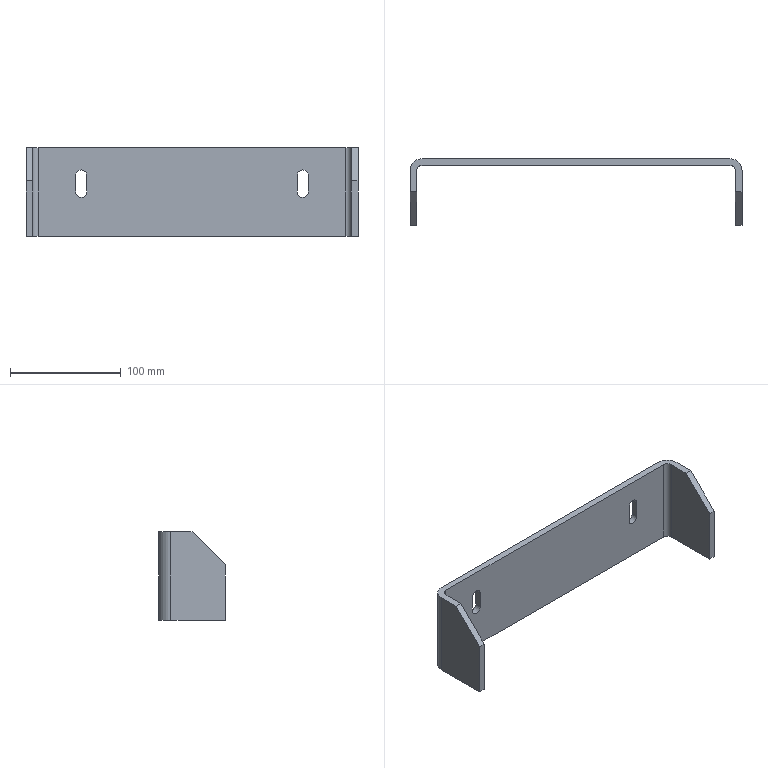Part | STEP file | VD-SYL0380DJ1006_1_1-12_VD-SYL0 | 1 solid | 26 faces | box 300 x 60 x 80 mm | volume 184401 mm3 | plane 16 | cylinder 10 | commonest cylinder face diameters 10 x8 22 x2
STEP:
#1=CARTESIAN_POINT('',(-105.,24.,15.));
#2=VERTEX_POINT('',#1);
#3=CARTESIAN_POINT('',(-100.,24.,20.));
#4=VERTEX_POINT('',#3);
#5=CARTESIAN_POINT('',(-100.,24.,15.));
#6=DIRECTION('',(0.,1.,0.));
#7=DIRECTION('',(-1.,0.,0.));
#8=AXIS2_PLACEMENT_3D('',#5,#6,#7);
#9=CIRCLE('',#8,5.);
#10=EDGE_CURVE('',#2,#4,#9,.T.);
#11=ORIENTED_EDGE('',*,*,#10,.F.);
#12=CARTESIAN_POINT('',(-105.,30.,15.));
#13=VERTEX_POINT('',#12);
#14=CARTESIAN_POINT('',(-105.,24.,15.));
#15=DIRECTION('',(0.,1.,0.));
#16=VECTOR('',#15,1000.);
#17=LINE('',#14,#16);
#18=EDGE_CURVE('',#2,#13,#17,.T.);
#19=ORIENTED_EDGE('',*,*,#18,.T.);
#20=CARTESIAN_POINT('',(-100.,30.,20.));
#21=VERTEX_POINT('',#20);
#22=CARTESIAN_POINT('',(-100.,30.,15.));
#23=DIRECTION('',(0.,-1.,0.));
#24=DIRECTION('',(0.,0.,1.));
#25=AXIS2_PLACEMENT_3D('',#22,#23,#24);
#26=CIRCLE('',#25,5.);
#27=EDGE_CURVE('',#21,#13,#26,.T.);
#28=ORIENTED_EDGE('',*,*,#27,.F.);
#29=CARTESIAN_POINT('',(-100.,30.,20.));
#30=DIRECTION('',(0.,-1.,0.));
#31=VECTOR('',#30,1000.);
#32=LINE('',#29,#31);
#33=EDGE_CURVE('',#21,#4,#32,.T.);
#34=ORIENTED_EDGE('',*,*,#33,.T.);
#35=EDGE_LOOP('',(#11,#19,#28,#34));
#36=FACE_OUTER_BOUND('',#35,.T.);
#37=CARTESIAN_POINT('',(-100.,27.,15.));
#38=DIRECTION('',(0.,1.,0.));
#39=DIRECTION('',(0.,0.,1.));
#40=AXIS2_PLACEMENT_3D('',#37,#38,#39);
#41=CYLINDRICAL_SURFACE('',#40,5.);
#42=ADVANCED_FACE('',(#36),#41,.F.);
#43=ORIENTED_EDGE('',*,*,#33,.F.);
#44=CARTESIAN_POINT('',(-95.,30.,15.));
#45=VERTEX_POINT('',#44);
#46=CARTESIAN_POINT('',(-100.,30.,15.));
#47=DIRECTION('',(0.,-1.,0.));
#48=DIRECTION('',(1.,0.,0.));
#49=AXIS2_PLACEMENT_3D('',#46,#47,#48);
#50=CIRCLE('',#49,5.);
#51=EDGE_CURVE('',#45,#21,#50,.T.);
#52=ORIENTED_EDGE('',*,*,#51,.F.);
#53=CARTESIAN_POINT('',(-95.,24.,15.));
#54=VERTEX_POINT('',#53);
#55=CARTESIAN_POINT('',(-95.,30.,15.));
#56=DIRECTION('',(0.,-1.,0.));
#57=VECTOR('',#56,1000.);
#58=LINE('',#55,#57);
#59=EDGE_CURVE('',#45,#54,#58,.T.);
#60=ORIENTED_EDGE('',*,*,#59,.T.);
#61=CARTESIAN_POINT('',(-100.,24.,15.));
#62=DIRECTION('',(0.,1.,0.));
#63=DIRECTION('',(0.,0.,1.));
#64=AXIS2_PLACEMENT_3D('',#61,#62,#63);
#65=CIRCLE('',#64,5.);
#66=EDGE_CURVE('',#4,#54,#65,.T.);
#67=ORIENTED_EDGE('',*,*,#66,.F.);
#68=EDGE_LOOP('',(#43,#52,#60,#67));
#69=FACE_OUTER_BOUND('',#68,.T.);
#70=CARTESIAN_POINT('',(-100.,27.,15.));
#71=DIRECTION('',(0.,1.,0.));
#72=DIRECTION('',(0.,0.,1.));
#73=AXIS2_PLACEMENT_3D('',#70,#71,#72);
#74=CYLINDRICAL_SURFACE('',#73,5.);
#75=ADVANCED_FACE('',(#69),#74,.F.);
#76=CARTESIAN_POINT('',(-95.,30.,0.));
#77=VERTEX_POINT('',#76);
#78=CARTESIAN_POINT('',(-95.,30.,15.));
#79=DIRECTION('',(0.,0.,-1.));
#80=VECTOR('',#79,1000.);
#81=LINE('',#78,#80);
#82=EDGE_CURVE('',#45,#77,#81,.T.);
#83=ORIENTED_EDGE('',*,*,#82,.T.);
#84=CARTESIAN_POINT('',(-95.,24.,0.));
#85=VERTEX_POINT('',#84);
#86=CARTESIAN_POINT('',(-95.,24.,0.));
#87=DIRECTION('',(0.,1.,0.));
#88=VECTOR('',#87,1000.);
#89=LINE('',#86,#88);
#90=EDGE_CURVE('',#85,#77,#89,.T.);
#91=ORIENTED_EDGE('',*,*,#90,.F.);
#92=CARTESIAN_POINT('',(-95.,24.,15.));
#93=DIRECTION('',(0.,0.,-1.));
#94=VECTOR('',#93,1000.);
#95=LINE('',#92,#94);
#96=EDGE_CURVE('',#54,#85,#95,.T.);
#97=ORIENTED_EDGE('',*,*,#96,.F.);
#98=ORIENTED_EDGE('',*,*,#59,.F.);
#99=EDGE_LOOP('',(#83,#91,#97,#98));
#100=FACE_OUTER_BOUND('',#99,.T.);
#101=CARTESIAN_POINT('',(-95.,27.,7.5));
#102=DIRECTION('',(-1.,0.,0.));
#103=DIRECTION('',(0.,0.,1.));
#104=AXIS2_PLACEMENT_3D('',#101,#102,#103);
#105=PLANE('',#104);
#106=ADVANCED_FACE('',(#100),#105,.T.);
#107=CARTESIAN_POINT('',(-105.,24.,0.));
#108=VERTEX_POINT('',#107);
#109=CARTESIAN_POINT('',(-100.,24.,0.));
#110=DIRECTION('',(0.,1.,0.));
#111=DIRECTION('',(1.,0.,0.));
#112=AXIS2_PLACEMENT_3D('',#109,#110,#111);
#113=CIRCLE('',#112,5.);
#114=EDGE_CURVE('',#85,#108,#113,.T.);
#115=ORIENTED_EDGE('',*,*,#114,.F.);
#116=ORIENTED_EDGE('',*,*,#90,.T.);
#117=CARTESIAN_POINT('',(-105.,30.,0.));
#118=VERTEX_POINT('',#117);
#119=CARTESIAN_POINT('',(-100.,30.,0.));
#120=DIRECTION('',(0.,-1.,0.));
#121=DIRECTION('',(-1.,0.,0.));
#122=AXIS2_PLACEMENT_3D('',#119,#120,#121);
#123=CIRCLE('',#122,5.);
#124=EDGE_CURVE('',#118,#77,#123,.T.);
#125=ORIENTED_EDGE('',*,*,#124,.F.);
#126=CARTESIAN_POINT('',(-105.,30.,0.));
#127=DIRECTION('',(0.,-1.,0.));
#128=VECTOR('',#127,1000.);
#129=LINE('',#126,#128);
#130=EDGE_CURVE('',#118,#108,#129,.T.);
#131=ORIENTED_EDGE('',*,*,#130,.T.);
#132=EDGE_LOOP('',(#115,#116,#125,#131));
#133=FACE_OUTER_BOUND('',#132,.T.);
#134=CARTESIAN_POINT('',(-100.,27.,0.));
#135=DIRECTION('',(0.,1.,0.));
#136=DIRECTION('',(0.,0.,1.));
#137=AXIS2_PLACEMENT_3D('',#134,#135,#136);
#138=CYLINDRICAL_SURFACE('',#137,5.);
#139=ADVANCED_FACE('',(#133),#138,.F.);
#140=CARTESIAN_POINT('',(-105.,30.,0.));
#141=DIRECTION('',(0.,0.,1.));
#142=VECTOR('',#141,1000.);
#143=LINE('',#140,#142);
#144=EDGE_CURVE('',#118,#13,#143,.T.);
#145=ORIENTED_EDGE('',*,*,#144,.T.);
#146=ORIENTED_EDGE('',*,*,#18,.F.);
#147=CARTESIAN_POINT('',(-105.,24.,0.));
#148=DIRECTION('',(0.,0.,1.));
#149=VECTOR('',#148,1000.);
#150=LINE('',#147,#149);
#151=EDGE_CURVE('',#108,#2,#150,.T.);
#152=ORIENTED_EDGE('',*,*,#151,.F.);
#153=ORIENTED_EDGE('',*,*,#130,.F.);
#154=EDGE_LOOP('',(#145,#146,#152,#153));
#155=FACE_OUTER_BOUND('',#154,.T.);
#156=CARTESIAN_POINT('',(-105.,27.,7.5));
#157=DIRECTION('',(1.,0.,0.));
#158=DIRECTION('',(0.,1.,0.));
#159=AXIS2_PLACEMENT_3D('',#156,#157,#158);
#160=PLANE('',#159);
#161=ADVANCED_FACE('',(#155),#160,.T.);
#162=CARTESIAN_POINT('',(105.,30.,15.));
#163=VERTEX_POINT('',#162);
#164=CARTESIAN_POINT('',(105.,30.,0.));
#165=VERTEX_POINT('',#164);
#166=CARTESIAN_POINT('',(105.,30.,15.));
#167=DIRECTION('',(0.,0.,-1.));
#168=VECTOR('',#167,1000.);
#169=LINE('',#166,#168);
#170=EDGE_CURVE('',#163,#165,#169,.T.);
#171=ORIENTED_EDGE('',*,*,#170,.T.);
#172=CARTESIAN_POINT('',(105.,24.,0.));
#173=VERTEX_POINT('',#172);
#174=CARTESIAN_POINT('',(105.,24.,0.));
#175=DIRECTION('',(0.,1.,0.));
#176=VECTOR('',#175,1000.);
#177=LINE('',#174,#176);
#178=EDGE_CURVE('',#173,#165,#177,.T.);
#179=ORIENTED_EDGE('',*,*,#178,.F.);
#180=CARTESIAN_POINT('',(105.,24.,15.));
#181=VERTEX_POINT('',#180);
#182=CARTESIAN_POINT('',(105.,24.,15.));
#183=DIRECTION('',(0.,0.,-1.));
#184=VECTOR('',#183,1000.);
#185=LINE('',#182,#184);
#186=EDGE_CURVE('',#181,#173,#185,.T.);
#187=ORIENTED_EDGE('',*,*,#186,.F.);
#188=CARTESIAN_POINT('',(105.,30.,15.));
#189=DIRECTION('',(0.,-1.,0.));
#190=VECTOR('',#189,1000.);
#191=LINE('',#188,#190);
#192=EDGE_CURVE('',#163,#181,#191,.T.);
#193=ORIENTED_EDGE('',*,*,#192,.F.);
#194=EDGE_LOOP('',(#171,#179,#187,#193));
#195=FACE_OUTER_BOUND('',#194,.T.);
#196=CARTESIAN_POINT('',(105.,27.,7.5));
#197=DIRECTION('',(-1.,0.,0.));
#198=DIRECTION('',(0.,0.,1.));
#199=AXIS2_PLACEMENT_3D('',#196,#197,#198);
#200=PLANE('',#199);
#201=ADVANCED_FACE('',(#195),#200,.T.);
#202=CARTESIAN_POINT('',(100.,30.,20.));
#203=VERTEX_POINT('',#202);
#204=CARTESIAN_POINT('',(100.,24.,20.));
#205=VERTEX_POINT('',#204);
#206=CARTESIAN_POINT('',(100.,30.,20.));
#207=DIRECTION('',(0.,-1.,0.));
#208=VECTOR('',#207,1000.);
#209=LINE('',#206,#208);
#210=EDGE_CURVE('',#203,#205,#209,.T.);
#211=ORIENTED_EDGE('',*,*,#210,.F.);
#212=CARTESIAN_POINT('',(100.,30.,15.));
#213=DIRECTION('',(0.,-1.,0.));
#214=DIRECTION('',(1.,0.,0.));
#215=AXIS2_PLACEMENT_3D('',#212,#213,#214);
#216=CIRCLE('',#215,5.);
#217=EDGE_CURVE('',#163,#203,#216,.T.);
#218=ORIENTED_EDGE('',*,*,#217,.F.);
#219=ORIENTED_EDGE('',*,*,#192,.T.);
#220=CARTESIAN_POINT('',(100.,24.,15.));
#221=DIRECTION('',(0.,1.,0.));
#222=DIRECTION('',(0.,0.,1.));
#223=AXIS2_PLACEMENT_3D('',#220,#221,#222);
#224=CIRCLE('',#223,5.);
#225=EDGE_CURVE('',#205,#181,#224,.T.);
#226=ORIENTED_EDGE('',*,*,#225,.F.);
#227=EDGE_LOOP('',(#211,#218,#219,#226));
#228=FACE_OUTER_BOUND('',#227,.T.);
#229=CARTESIAN_POINT('',(100.,27.,15.));
#230=DIRECTION('',(0.,1.,0.));
#231=DIRECTION('',(0.,0.,1.));
#232=AXIS2_PLACEMENT_3D('',#229,#230,#231);
#233=CYLINDRICAL_SURFACE('',#232,5.);
#234=ADVANCED_FACE('',(#228),#233,.F.);
#235=CARTESIAN_POINT('',(95.,24.,15.));
#236=VERTEX_POINT('',#235);
#237=CARTESIAN_POINT('',(100.,24.,15.));
#238=DIRECTION('',(0.,1.,0.));
#239=DIRECTION('',(-1.,0.,0.));
#240=AXIS2_PLACEMENT_3D('',#237,#238,#239);
#241=CIRCLE('',#240,5.);
#242=EDGE_CURVE('',#236,#205,#241,.T.);
#243=ORIENTED_EDGE('',*,*,#242,.F.);
#244=CARTESIAN_POINT('',(95.,30.,15.));
#245=VERTEX_POINT('',#244);
#246=CARTESIAN_POINT('',(95.,24.,15.));
#247=DIRECTION('',(0.,1.,0.));
#248=VECTOR('',#247,1000.);
#249=LINE('',#246,#248);
#250=EDGE_CURVE('',#236,#245,#249,.T.);
#251=ORIENTED_EDGE('',*,*,#250,.T.);
#252=CARTESIAN_POINT('',(100.,30.,15.));
#253=DIRECTION('',(0.,-1.,0.));
#254=DIRECTION('',(0.,0.,1.));
#255=AXIS2_PLACEMENT_3D('',#252,#253,#254);
#256=CIRCLE('',#255,5.);
#257=EDGE_CURVE('',#203,#245,#256,.T.);
#258=ORIENTED_EDGE('',*,*,#257,.F.);
#259=ORIENTED_EDGE('',*,*,#210,.T.);
#260=EDGE_LOOP('',(#243,#251,#258,#259));
#261=FACE_OUTER_BOUND('',#260,.T.);
#262=CARTESIAN_POINT('',(100.,27.,15.));
#263=DIRECTION('',(0.,1.,0.));
#264=DIRECTION('',(0.,0.,1.));
#265=AXIS2_PLACEMENT_3D('',#262,#263,#264);
#266=CYLINDRICAL_SURFACE('',#265,5.);
#267=ADVANCED_FACE('',(#261),#266,.F.);
#268=CARTESIAN_POINT('',(-139.,24.,-40.));
#269=VERTEX_POINT('',#268);
#270=CARTESIAN_POINT('',(-144.,19.,-40.));
#271=VERTEX_POINT('',#270);
#272=CARTESIAN_POINT('',(-139.,19.,-40.));
#273=DIRECTION('',(0.,0.,1.));
#274=DIRECTION('',(0.,1.,0.));
#275=AXIS2_PLACEMENT_3D('',#272,#273,#274);
#276=CIRCLE('',#275,5.);
#277=EDGE_CURVE('',#269,#271,#276,.T.);
#278=ORIENTED_EDGE('',*,*,#277,.F.);
#279=CARTESIAN_POINT('',(-139.,24.,40.));
#280=VERTEX_POINT('',#279);
#281=CARTESIAN_POINT('',(-139.,24.,-40.));
#282=DIRECTION('',(0.,0.,1.));
#283=VECTOR('',#282,1000.);
#284=LINE('',#281,#283);
#285=EDGE_CURVE('',#269,#280,#284,.T.);
#286=ORIENTED_EDGE('',*,*,#285,.T.);
#287=CARTESIAN_POINT('',(-144.,19.,40.));
#288=VERTEX_POINT('',#287);
#289=CARTESIAN_POINT('',(-139.,19.,40.));
#290=DIRECTION('',(0.,0.,-1.));
#291=DIRECTION('',(-1.,0.,0.));
#292=AXIS2_PLACEMENT_3D('',#289,#290,#291);
#293=CIRCLE('',#292,5.);
#294=EDGE_CURVE('',#288,#280,#293,.T.);
#295=ORIENTED_EDGE('',*,*,#294,.F.);
#296=CARTESIAN_POINT('',(-144.,19.,40.));
#297=DIRECTION('',(0.,0.,-1.));
#298=VECTOR('',#297,1000.);
#299=LINE('',#296,#298);
#300=EDGE_CURVE('',#288,#271,#299,.T.);
#301=ORIENTED_EDGE('',*,*,#300,.T.);
#302=EDGE_LOOP('',(#278,#286,#295,#301));
#303=FACE_OUTER_BOUND('',#302,.T.);
#304=CARTESIAN_POINT('',(-139.,19.,350.437));
#305=DIRECTION('',(0.,0.,-1.));
#306=DIRECTION('',(-1.,0.,0.));
#307=AXIS2_PLACEMENT_3D('',#304,#305,#306);
#308=CYLINDRICAL_SURFACE('',#307,5.);
#309=ADVANCED_FACE('',(#303),#308,.F.);
#310=CARTESIAN_POINT('',(-150.,-30.,10.));
#311=VERTEX_POINT('',#310);
#312=CARTESIAN_POINT('',(-150.,0.,40.));
#313=VERTEX_POINT('',#312);
#314=CARTESIAN_POINT('',(-150.,-30.,10.));
#315=DIRECTION('',(0.,0.7071,0.7071));
#316=VECTOR('',#315,1000.);
#317=LINE('',#314,#316);
#318=EDGE_CURVE('',#311,#313,#317,.T.);
#319=ORIENTED_EDGE('',*,*,#318,.F.);
#320=CARTESIAN_POINT('',(-144.,-30.,10.));
#321=VERTEX_POINT('',#320);
#322=CARTESIAN_POINT('',(-144.,-30.,10.));
#323=DIRECTION('',(-1.,0.,0.));
#324=VECTOR('',#323,1000.);
#325=LINE('',#322,#324);
#326=EDGE_CURVE('',#321,#311,#325,.T.);
#327=ORIENTED_EDGE('',*,*,#326,.F.);
#328=CARTESIAN_POINT('',(-144.,0.,40.));
#329=VERTEX_POINT('',#328);
#330=CARTESIAN_POINT('',(-144.,0.,40.));
#331=DIRECTION('',(0.,-0.7071,-0.7071));
#332=VECTOR('',#331,1000.);
#333=LINE('',#330,#332);
#334=EDGE_CURVE('',#329,#321,#333,.T.);
#335=ORIENTED_EDGE('',*,*,#334,.F.);
#336=CARTESIAN_POINT('',(-150.,0.,40.));
#337=DIRECTION('',(1.,0.,0.));
#338=VECTOR('',#337,1000.);
#339=LINE('',#336,#338);
#340=EDGE_CURVE('',#313,#329,#339,.T.);
#341=ORIENTED_EDGE('',*,*,#340,.F.);
#342=EDGE_LOOP('',(#319,#327,#335,#341));
#343=FACE_OUTER_BOUND('',#342,.T.);
#344=CARTESIAN_POINT('',(-147.,-15.,25.));
#345=DIRECTION('',(0.,-0.7071,0.7071));
#346=DIRECTION('',(-1.,0.,0.));
#347=AXIS2_PLACEMENT_3D('',#344,#345,#346);
#348=PLANE('',#347);
#349=ADVANCED_FACE('',(#343),#348,.T.);
#350=ORIENTED_EDGE('',*,*,#300,.F.);
#351=CARTESIAN_POINT('',(-144.,0.,40.));
#352=DIRECTION('',(0.,1.,0.));
#353=VECTOR('',#352,1000.);
#354=LINE('',#351,#353);
#355=EDGE_CURVE('',#329,#288,#354,.T.);
#356=ORIENTED_EDGE('',*,*,#355,.F.);
#357=ORIENTED_EDGE('',*,*,#334,.T.);
#358=CARTESIAN_POINT('',(-144.,-30.,-40.));
#359=VERTEX_POINT('',#358);
#360=CARTESIAN_POINT('',(-144.,-30.,10.));
#361=DIRECTION('',(0.,0.,-1.));
#362=VECTOR('',#361,1000.);
#363=LINE('',#360,#362);
#364=EDGE_CURVE('',#321,#359,#363,.T.);
#365=ORIENTED_EDGE('',*,*,#364,.T.);
#366=CARTESIAN_POINT('',(-144.,-30.,-40.));
#367=DIRECTION('',(0.,1.,0.));
#368=VECTOR('',#367,1000.);
#369=LINE('',#366,#368);
#370=EDGE_CURVE('',#359,#271,#369,.T.);
#371=ORIENTED_EDGE('',*,*,#370,.T.);
#372=EDGE_LOOP('',(#350,#356,#357,#365,#371));
#373=FACE_OUTER_BOUND('',#372,.T.);
#374=CARTESIAN_POINT('',(-144.,30.,-40.));
#375=DIRECTION('',(-1.,0.,0.));
#376=DIRECTION('',(0.,0.,1.));
#377=AXIS2_PLACEMENT_3D('',#374,#375,#376);
#378=PLANE('',#377);
#379=ADVANCED_FACE('',(#373),#378,.F.);
#380=ORIENTED_EDGE('',*,*,#326,.T.);
#381=CARTESIAN_POINT('',(-150.,-30.,-40.));
#382=VERTEX_POINT('',#381);
#383=CARTESIAN_POINT('',(-150.,-30.,10.));
#384=DIRECTION('',(0.,0.,-1.));
#385=VECTOR('',#384,1000.);
#386=LINE('',#383,#385);
#387=EDGE_CURVE('',#311,#382,#386,.T.);
#388=ORIENTED_EDGE('',*,*,#387,.T.);
#389=CARTESIAN_POINT('',(-144.,-30.,-40.));
#390=DIRECTION('',(-1.,0.,0.));
#391=VECTOR('',#390,1000.);
#392=LINE('',#389,#391);
#393=EDGE_CURVE('',#359,#382,#392,.T.);
#394=ORIENTED_EDGE('',*,*,#393,.F.);
#395=ORIENTED_EDGE('',*,*,#364,.F.);
#396=EDGE_LOOP('',(#380,#388,#394,#395));
#397=FACE_OUTER_BOUND('',#396,.T.);
#398=CARTESIAN_POINT('',(-147.,-30.,0.));
#399=DIRECTION('',(0.,-1.,0.));
#400=DIRECTION('',(0.,0.,-1.));
#401=AXIS2_PLACEMENT_3D('',#398,#399,#400);
#402=PLANE('',#401);
#403=ADVANCED_FACE('',(#397),#402,.T.);
#404=ORIENTED_EDGE('',*,*,#318,.T.);
#405=CARTESIAN_POINT('',(-150.,19.,40.));
#406=VERTEX_POINT('',#405);
#407=CARTESIAN_POINT('',(-150.,19.,40.));
#408=DIRECTION('',(0.,-1.,0.));
#409=VECTOR('',#408,1000.);
#410=LINE('',#407,#409);
#411=EDGE_CURVE('',#406,#313,#410,.T.);
#412=ORIENTED_EDGE('',*,*,#411,.F.);
#413=CARTESIAN_POINT('',(-150.,19.,-40.));
#414=VERTEX_POINT('',#413);
#415=CARTESIAN_POINT('',(-150.,19.,-40.));
#416=DIRECTION('',(0.,0.,1.));
#417=VECTOR('',#416,1000.);
#418=LINE('',#415,#417);
#419=EDGE_CURVE('',#414,#406,#418,.T.);
#420=ORIENTED_EDGE('',*,*,#419,.F.);
#421=CARTESIAN_POINT('',(-150.,-30.,-40.));
#422=DIRECTION('',(0.,1.,0.));
#423=VECTOR('',#422,1000.);
#424=LINE('',#421,#423);
#425=EDGE_CURVE('',#382,#414,#424,.T.);
#426=ORIENTED_EDGE('',*,*,#425,.F.);
#427=ORIENTED_EDGE('',*,*,#387,.F.);
#428=EDGE_LOOP('',(#404,#412,#420,#426,#427));
#429=FACE_OUTER_BOUND('',#428,.T.);
#430=CARTESIAN_POINT('',(-150.,30.,-40.));
#431=DIRECTION('',(-1.,0.,0.));
#432=DIRECTION('',(0.,0.,1.));
#433=AXIS2_PLACEMENT_3D('',#430,#431,#432);
#434=PLANE('',#433);
#435=ADVANCED_FACE('',(#429),#434,.T.);
#436=CARTESIAN_POINT('',(-139.,30.,40.));
#437=VERTEX_POINT('',#436);
#438=CARTESIAN_POINT('',(-139.,30.,-40.));
#439=VERTEX_POINT('',#438);
#440=CARTESIAN_POINT('',(-139.,30.,40.));
#441=DIRECTION('',(0.,0.,-1.));
#442=VECTOR('',#441,1000.);
#443=LINE('',#440,#442);
#444=EDGE_CURVE('',#437,#439,#443,.T.);
#445=ORIENTED_EDGE('',*,*,#444,.T.);
#446=CARTESIAN_POINT('',(-139.,19.,-40.));
#447=DIRECTION('',(0.,0.,-1.));
#448=DIRECTION('',(-1.,0.,0.));
#449=AXIS2_PLACEMENT_3D('',#446,#447,#448);
#450=CIRCLE('',#449,11.);
#451=EDGE_CURVE('',#414,#439,#450,.T.);
#452=ORIENTED_EDGE('',*,*,#451,.F.);
#453=ORIENTED_EDGE('',*,*,#419,.T.);
#454=CARTESIAN_POINT('',(-139.,19.,40.));
#455=DIRECTION('',(0.,0.,1.));
#456=DIRECTION('',(0.,1.,0.));
#457=AXIS2_PLACEMENT_3D('',#454,#455,#456);
#458=CIRCLE('',#457,11.);
#459=EDGE_CURVE('',#437,#406,#458,.T.);
#460=ORIENTED_EDGE('',*,*,#459,.F.);
#461=EDGE_LOOP('',(#445,#452,#453,#460));
#462=FACE_OUTER_BOUND('',#461,.T.);
#463=CARTESIAN_POINT('',(-139.,19.,350.437));
#464=DIRECTION('',(0.,0.,-1.));
#465=DIRECTION('',(-1.,0.,0.));
#466=AXIS2_PLACEMENT_3D('',#463,#464,#465);
#467=CYLINDRICAL_SURFACE('',#466,11.);
#468=ADVANCED_FACE('',(#462),#467,.T.);
#469=CARTESIAN_POINT('',(150.,19.,40.));
#470=VERTEX_POINT('',#469);
#471=CARTESIAN_POINT('',(150.,19.,-40.));
#472=VERTEX_POINT('',#471);
#473=CARTESIAN_POINT('',(150.,19.,40.));
#474=DIRECTION('',(0.,0.,-1.));
#475=VECTOR('',#474,1000.);
#476=LINE('',#473,#475);
#477=EDGE_CURVE('',#470,#472,#476,.T.);
#478=ORIENTED_EDGE('',*,*,#477,.T.);
#479=CARTESIAN_POINT('',(139.,30.,-40.));
#480=VERTEX_POINT('',#479);
#481=CARTESIAN_POINT('',(139.,19.,-40.));
#482=DIRECTION('',(0.,0.,-1.));
#483=DIRECTION('',(0.,1.,0.));
#484=AXIS2_PLACEMENT_3D('',#481,#482,#483);
#485=CIRCLE('',#484,11.);
#486=EDGE_CURVE('',#480,#472,#485,.T.);
#487=ORIENTED_EDGE('',*,*,#486,.F.);
#488=CARTESIAN_POINT('',(139.,30.,40.));
#489=VERTEX_POINT('',#488);
#490=CARTESIAN_POINT('',(139.,30.,-40.));
#491=DIRECTION('',(0.,0.,1.));
#492=VECTOR('',#491,1000.);
#493=LINE('',#490,#492);
#494=EDGE_CURVE('',#480,#489,#493,.T.);
#495=ORIENTED_EDGE('',*,*,#494,.T.);
#496=CARTESIAN_POINT('',(139.,19.,40.));
#497=DIRECTION('',(0.,0.,1.));
#498=DIRECTION('',(1.,0.,0.));
#499=AXIS2_PLACEMENT_3D('',#496,#497,#498);
#500=CIRCLE('',#499,11.);
#501=EDGE_CURVE('',#470,#489,#500,.T.);
#502=ORIENTED_EDGE('',*,*,#501,.F.);
#503=EDGE_LOOP('',(#478,#487,#495,#502));
#504=FACE_OUTER_BOUND('',#503,.T.);
#505=CARTESIAN_POINT('',(139.,19.,350.437));
#506=DIRECTION('',(0.,0.,-1.));
#507=DIRECTION('',(-1.,0.,0.));
#508=AXIS2_PLACEMENT_3D('',#505,#506,#507);
#509=CYLINDRICAL_SURFACE('',#508,11.);
#510=ADVANCED_FACE('',(#504),#509,.T.);
#511=CARTESIAN_POINT('',(150.,0.,40.));
#512=VERTEX_POINT('',#511);
#513=CARTESIAN_POINT('',(150.,-30.,10.));
#514=VERTEX_POINT('',#513);
#515=CARTESIAN_POINT('',(150.,0.,40.));
#516=DIRECTION('',(0.,-0.7071,-0.7071));
#517=VECTOR('',#516,1000.);
#518=LINE('',#515,#517);
#519=EDGE_CURVE('',#512,#514,#518,.T.);
#520=ORIENTED_EDGE('',*,*,#519,.T.);
#521=CARTESIAN_POINT('',(150.,-30.,-40.));
#522=VERTEX_POINT('',#521);
#523=CARTESIAN_POINT('',(150.,-30.,-40.));
#524=DIRECTION('',(0.,0.,1.));
#525=VECTOR('',#524,1000.);
#526=LINE('',#523,#525);
#527=EDGE_CURVE('',#522,#514,#526,.T.);
#528=ORIENTED_EDGE('',*,*,#527,.F.);
#529=CARTESIAN_POINT('',(150.,19.,-40.));
#530=DIRECTION('',(0.,-1.,0.));
#531=VECTOR('',#530,1000.);
#532=LINE('',#529,#531);
#533=EDGE_CURVE('',#472,#522,#532,.T.);
#534=ORIENTED_EDGE('',*,*,#533,.F.);
#535=ORIENTED_EDGE('',*,*,#477,.F.);
#536=CARTESIAN_POINT('',(150.,0.,40.));
#537=DIRECTION('',(0.,1.,0.));
#538=VECTOR('',#537,1000.);
#539=LINE('',#536,#538);
#540=EDGE_CURVE('',#512,#470,#539,.T.);
#541=ORIENTED_EDGE('',*,*,#540,.F.);
#542=EDGE_LOOP('',(#520,#528,#534,#535,#541));
#543=FACE_OUTER_BOUND('',#542,.T.);
#544=CARTESIAN_POINT('',(150.,-30.,-40.));
#545=DIRECTION('',(1.,0.,0.));
#546=DIRECTION('',(0.,1.,0.));
#547=AXIS2_PLACEMENT_3D('',#544,#545,#546);
#548=PLANE('',#547);
#549=ADVANCED_FACE('',(#543),#548,.T.);
#550=ORIENTED_EDGE('',*,*,#527,.T.);
#551=CARTESIAN_POINT('',(144.,-30.,10.));
#552=VERTEX_POINT('',#551);
#553=CARTESIAN_POINT('',(150.,-30.,10.));
#554=DIRECTION('',(-1.,0.,0.));
#555=VECTOR('',#554,1000.);
#556=LINE('',#553,#555);
#557=EDGE_CURVE('',#514,#552,#556,.T.);
#558=ORIENTED_EDGE('',*,*,#557,.T.);
#559=CARTESIAN_POINT('',(144.,-30.,-40.));
#560=VERTEX_POINT('',#559);
#561=CARTESIAN_POINT('',(144.,-30.,10.));
#562=DIRECTION('',(0.,0.,-1.));
#563=VECTOR('',#562,1000.);
#564=LINE('',#561,#563);
#565=EDGE_CURVE('',#552,#560,#564,.T.);
#566=ORIENTED_EDGE('',*,*,#565,.T.);
#567=CARTESIAN_POINT('',(144.,-30.,-40.));
#568=DIRECTION('',(1.,0.,0.));
#569=VECTOR('',#568,1000.);
#570=LINE('',#567,#569);
#571=EDGE_CURVE('',#560,#522,#570,.T.);
#572=ORIENTED_EDGE('',*,*,#571,.T.);
#573=EDGE_LOOP('',(#550,#558,#566,#572));
#574=FACE_OUTER_BOUND('',#573,.T.);
#575=CARTESIAN_POINT('',(147.,-30.,0.));
#576=DIRECTION('',(0.,1.,0.));
#577=DIRECTION('',(1.,0.,0.));
#578=AXIS2_PLACEMENT_3D('',#575,#576,#577);
#579=PLANE('',#578);
#580=ADVANCED_FACE('',(#574),#579,.F.);
#581=ORIENTED_EDGE('',*,*,#519,.F.);
#582=CARTESIAN_POINT('',(144.,0.,40.));
#583=VERTEX_POINT('',#582);
#584=CARTESIAN_POINT('',(144.,0.,40.));
#585=DIRECTION('',(1.,0.,0.));
#586=VECTOR('',#585,1000.);
#587=LINE('',#584,#586);
#588=EDGE_CURVE('',#583,#512,#587,.T.);
#589=ORIENTED_EDGE('',*,*,#588,.F.);
#590=CARTESIAN_POINT('',(144.,-30.,10.));
#591=DIRECTION('',(0.,0.7071,0.7071));
#592=VECTOR('',#591,1000.);
#593=LINE('',#590,#592);
#594=EDGE_CURVE('',#552,#583,#593,.T.);
#595=ORIENTED_EDGE('',*,*,#594,.F.);
#596=ORIENTED_EDGE('',*,*,#557,.F.);
#597=EDGE_LOOP('',(#581,#589,#595,#596));
#598=FACE_OUTER_BOUND('',#597,.T.);
#599=CARTESIAN_POINT('',(147.,-15.,25.));
#600=DIRECTION('',(0.,-0.7071,0.7071));
#601=DIRECTION('',(-1.,0.,0.));
#602=AXIS2_PLACEMENT_3D('',#599,#600,#601);
#603=PLANE('',#602);
#604=ADVANCED_FACE('',(#598),#603,.T.);
#605=CARTESIAN_POINT('',(144.,19.,-40.));
#606=VERTEX_POINT('',#605);
#607=CARTESIAN_POINT('',(144.,19.,-40.));
#608=DIRECTION('',(0.,-1.,0.));
#609=VECTOR('',#608,1000.);
#610=LINE('',#607,#609);
#611=EDGE_CURVE('',#606,#560,#610,.T.);
#612=ORIENTED_EDGE('',*,*,#611,.T.);
#613=ORIENTED_EDGE('',*,*,#565,.F.);
#614=ORIENTED_EDGE('',*,*,#594,.T.);
#615=CARTESIAN_POINT('',(144.,19.,40.));
#616=VERTEX_POINT('',#615);
#617=CARTESIAN_POINT('',(144.,19.,40.));
#618=DIRECTION('',(0.,-1.,0.));
#619=VECTOR('',#618,1000.);
#620=LINE('',#617,#619);
#621=EDGE_CURVE('',#616,#583,#620,.T.);
#622=ORIENTED_EDGE('',*,*,#621,.F.);
#623=CARTESIAN_POINT('',(144.,19.,-40.));
#624=DIRECTION('',(0.,0.,1.));
#625=VECTOR('',#624,1000.);
#626=LINE('',#623,#625);
#627=EDGE_CURVE('',#606,#616,#626,.T.);
#628=ORIENTED_EDGE('',*,*,#627,.F.);
#629=EDGE_LOOP('',(#612,#613,#614,#622,#628));
#630=FACE_OUTER_BOUND('',#629,.T.);
#631=CARTESIAN_POINT('',(144.,-30.,-40.));
#632=DIRECTION('',(1.,0.,0.));
#633=DIRECTION('',(0.,1.,0.));
#634=AXIS2_PLACEMENT_3D('',#631,#632,#633);
#635=PLANE('',#634);
#636=ADVANCED_FACE('',(#630),#635,.F.);
#637=ORIENTED_EDGE('',*,*,#277,.T.);
#638=ORIENTED_EDGE('',*,*,#370,.F.);
#639=ORIENTED_EDGE('',*,*,#393,.T.);
#640=ORIENTED_EDGE('',*,*,#425,.T.);
#641=ORIENTED_EDGE('',*,*,#451,.T.);
#642=CARTESIAN_POINT('',(-139.,30.,-40.));
#643=DIRECTION('',(1.,0.,0.));
#644=VECTOR('',#643,1000.);
#645=LINE('',#642,#644);
#646=EDGE_CURVE('',#439,#480,#645,.T.);
#647=ORIENTED_EDGE('',*,*,#646,.T.);
#648=ORIENTED_EDGE('',*,*,#486,.T.);
#649=ORIENTED_EDGE('',*,*,#533,.T.);
#650=ORIENTED_EDGE('',*,*,#571,.F.);
#651=ORIENTED_EDGE('',*,*,#611,.F.);
#652=CARTESIAN_POINT('',(139.,24.,-40.));
#653=VERTEX_POINT('',#652);
#654=CARTESIAN_POINT('',(139.,19.,-40.));
#655=DIRECTION('',(0.,0.,1.));
#656=DIRECTION('',(1.,0.,0.));
#657=AXIS2_PLACEMENT_3D('',#654,#655,#656);
#658=CIRCLE('',#657,5.);
#659=EDGE_CURVE('',#606,#653,#658,.T.);
#660=ORIENTED_EDGE('',*,*,#659,.T.);
#661=CARTESIAN_POINT('',(-139.,24.,-40.));
#662=DIRECTION('',(1.,0.,0.));
#663=VECTOR('',#662,1000.);
#664=LINE('',#661,#663);
#665=EDGE_CURVE('',#269,#653,#664,.T.);
#666=ORIENTED_EDGE('',*,*,#665,.F.);
#667=EDGE_LOOP('',(#637,#638,#639,#640,#641,#647,#648,#649,#650,#651,#660,#666));
#668=FACE_OUTER_BOUND('',#667,.T.);
#669=CARTESIAN_POINT('',(0.,27.,-40.));
#670=DIRECTION('',(0.,0.,-1.));
#671=DIRECTION('',(0.,-1.,0.));
#672=AXIS2_PLACEMENT_3D('',#669,#670,#671);
#673=PLANE('',#672);
#674=ADVANCED_FACE('',(#668),#673,.T.);
#675=ORIENTED_EDGE('',*,*,#124,.T.);
#676=ORIENTED_EDGE('',*,*,#82,.F.);
#677=ORIENTED_EDGE('',*,*,#51,.T.);
#678=ORIENTED_EDGE('',*,*,#27,.T.);
#679=ORIENTED_EDGE('',*,*,#144,.F.);
#680=EDGE_LOOP('',(#675,#676,#677,#678,#679));
#681=FACE_BOUND('',#680,.T.);
#682=CARTESIAN_POINT('',(95.,30.,0.));
#683=VERTEX_POINT('',#682);
#684=CARTESIAN_POINT('',(100.,30.,0.));
#685=DIRECTION('',(0.,-1.,0.));
#686=DIRECTION('',(0.,0.,-1.));
#687=AXIS2_PLACEMENT_3D('',#684,#685,#686);
#688=CIRCLE('',#687,5.);
#689=EDGE_CURVE('',#683,#165,#688,.T.);
#690=ORIENTED_EDGE('',*,*,#689,.T.);
#691=ORIENTED_EDGE('',*,*,#170,.F.);
#692=ORIENTED_EDGE('',*,*,#217,.T.);
#693=ORIENTED_EDGE('',*,*,#257,.T.);
#694=CARTESIAN_POINT('',(95.,30.,0.));
#695=DIRECTION('',(0.,0.,1.));
#696=VECTOR('',#695,1000.);
#697=LINE('',#694,#696);
#698=EDGE_CURVE('',#683,#245,#697,.T.);
#699=ORIENTED_EDGE('',*,*,#698,.F.);
#700=EDGE_LOOP('',(#690,#691,#692,#693,#699));
#701=FACE_BOUND('',#700,.T.);
#702=ORIENTED_EDGE('',*,*,#444,.F.);
#703=CARTESIAN_POINT('',(139.,30.,40.));
#704=DIRECTION('',(-1.,0.,0.));
#705=VECTOR('',#704,1000.);
#706=LINE('',#703,#705);
#707=EDGE_CURVE('',#489,#437,#706,.T.);
#708=ORIENTED_EDGE('',*,*,#707,.F.);
#709=ORIENTED_EDGE('',*,*,#494,.F.);
#710=ORIENTED_EDGE('',*,*,#646,.F.);
#711=EDGE_LOOP('',(#702,#708,#709,#710));
#712=FACE_OUTER_BOUND('',#711,.T.);
#713=CARTESIAN_POINT('',(150.,30.,-40.));
#714=DIRECTION('',(0.,1.,0.));
#715=DIRECTION('',(1.,0.,0.));
#716=AXIS2_PLACEMENT_3D('',#713,#714,#715);
#717=PLANE('',#716);
#718=ADVANCED_FACE('',(#681,#701,#712),#717,.T.);
#719=ORIENTED_EDGE('',*,*,#459,.T.);
#720=ORIENTED_EDGE('',*,*,#411,.T.);
#721=ORIENTED_EDGE('',*,*,#340,.T.);
#722=ORIENTED_EDGE('',*,*,#355,.T.);
#723=ORIENTED_EDGE('',*,*,#294,.T.);
#724=CARTESIAN_POINT('',(139.,24.,40.));
#725=VERTEX_POINT('',#724);
#726=CARTESIAN_POINT('',(-139.,24.,40.));
#727=DIRECTION('',(1.,0.,0.));
#728=VECTOR('',#727,1000.);
#729=LINE('',#726,#728);
#730=EDGE_CURVE('',#280,#725,#729,.T.);
#731=ORIENTED_EDGE('',*,*,#730,.T.);
#732=CARTESIAN_POINT('',(139.,19.,40.));
#733=DIRECTION('',(0.,0.,-1.));
#734=DIRECTION('',(0.,1.,0.));
#735=AXIS2_PLACEMENT_3D('',#732,#733,#734);
#736=CIRCLE('',#735,5.);
#737=EDGE_CURVE('',#725,#616,#736,.T.);
#738=ORIENTED_EDGE('',*,*,#737,.T.);
#739=ORIENTED_EDGE('',*,*,#621,.T.);
#740=ORIENTED_EDGE('',*,*,#588,.T.);
#741=ORIENTED_EDGE('',*,*,#540,.T.);
#742=ORIENTED_EDGE('',*,*,#501,.T.);
#743=ORIENTED_EDGE('',*,*,#707,.T.);
#744=EDGE_LOOP('',(#719,#720,#721,#722,#723,#731,#738,#739,#740,#741,#742,#743));
#745=FACE_OUTER_BOUND('',#744,.T.);
#746=CARTESIAN_POINT('',(0.,27.,40.));
#747=DIRECTION('',(0.,0.,-1.));
#748=DIRECTION('',(0.,-1.,0.));
#749=AXIS2_PLACEMENT_3D('',#746,#747,#748);
#750=PLANE('',#749);
#751=ADVANCED_FACE('',(#745),#750,.F.);
#752=ORIENTED_EDGE('',*,*,#659,.F.);
#753=ORIENTED_EDGE('',*,*,#627,.T.);
#754=ORIENTED_EDGE('',*,*,#737,.F.);
#755=CARTESIAN_POINT('',(139.,24.,40.));
#756=DIRECTION('',(0.,0.,-1.));
#757=VECTOR('',#756,1000.);
#758=LINE('',#755,#757);
#759=EDGE_CURVE('',#725,#653,#758,.T.);
#760=ORIENTED_EDGE('',*,*,#759,.T.);
#761=EDGE_LOOP('',(#752,#753,#754,#760));
#762=FACE_OUTER_BOUND('',#761,.T.);
#763=CARTESIAN_POINT('',(139.,19.,350.437));
#764=DIRECTION('',(0.,0.,-1.));
#765=DIRECTION('',(-1.,0.,0.));
#766=AXIS2_PLACEMENT_3D('',#763,#764,#765);
#767=CYLINDRICAL_SURFACE('',#766,5.);
#768=ADVANCED_FACE('',(#762),#767,.F.);
#769=ORIENTED_EDGE('',*,*,#242,.T.);
#770=ORIENTED_EDGE('',*,*,#225,.T.);
#771=ORIENTED_EDGE('',*,*,#186,.T.);
#772=CARTESIAN_POINT('',(95.,24.,0.));
#773=VERTEX_POINT('',#772);
#774=CARTESIAN_POINT('',(100.,24.,0.));
#775=DIRECTION('',(0.,1.,0.));
#776=DIRECTION('',(1.,0.,0.));
#777=AXIS2_PLACEMENT_3D('',#774,#775,#776);
#778=CIRCLE('',#777,5.);
#779=EDGE_CURVE('',#173,#773,#778,.T.);
#780=ORIENTED_EDGE('',*,*,#779,.T.);
#781=CARTESIAN_POINT('',(95.,24.,0.));
#782=DIRECTION('',(0.,0.,1.));
#783=VECTOR('',#782,1000.);
#784=LINE('',#781,#783);
#785=EDGE_CURVE('',#773,#236,#784,.T.);
#786=ORIENTED_EDGE('',*,*,#785,.T.);
#787=EDGE_LOOP('',(#769,#770,#771,#780,#786));
#788=FACE_BOUND('',#787,.T.);
#789=ORIENTED_EDGE('',*,*,#66,.T.);
#790=ORIENTED_EDGE('',*,*,#96,.T.);
#791=ORIENTED_EDGE('',*,*,#114,.T.);
#792=ORIENTED_EDGE('',*,*,#151,.T.);
#793=ORIENTED_EDGE('',*,*,#10,.T.);
#794=EDGE_LOOP('',(#789,#790,#791,#792,#793));
#795=FACE_BOUND('',#794,.T.);
#796=ORIENTED_EDGE('',*,*,#730,.F.);
#797=ORIENTED_EDGE('',*,*,#285,.F.);
#798=ORIENTED_EDGE('',*,*,#665,.T.);
#799=ORIENTED_EDGE('',*,*,#759,.F.);
#800=EDGE_LOOP('',(#796,#797,#798,#799));
#801=FACE_OUTER_BOUND('',#800,.T.);
#802=CARTESIAN_POINT('',(150.,24.,-40.));
#803=DIRECTION('',(0.,1.,0.));
#804=DIRECTION('',(1.,0.,0.));
#805=AXIS2_PLACEMENT_3D('',#802,#803,#804);
#806=PLANE('',#805);
#807=ADVANCED_FACE('',(#788,#795,#801),#806,.F.);
#808=ORIENTED_EDGE('',*,*,#779,.F.);
#809=ORIENTED_EDGE('',*,*,#178,.T.);
#810=ORIENTED_EDGE('',*,*,#689,.F.);
#811=CARTESIAN_POINT('',(95.,30.,0.));
#812=DIRECTION('',(0.,-1.,0.));
#813=VECTOR('',#812,1000.);
#814=LINE('',#811,#813);
#815=EDGE_CURVE('',#683,#773,#814,.T.);
#816=ORIENTED_EDGE('',*,*,#815,.T.);
#817=EDGE_LOOP('',(#808,#809,#810,#816));
#818=FACE_OUTER_BOUND('',#817,.T.);
#819=CARTESIAN_POINT('',(100.,27.,0.));
#820=DIRECTION('',(0.,1.,0.));
#821=DIRECTION('',(0.,0.,1.));
#822=AXIS2_PLACEMENT_3D('',#819,#820,#821);
#823=CYLINDRICAL_SURFACE('',#822,5.);
#824=ADVANCED_FACE('',(#818),#823,.F.);
#825=ORIENTED_EDGE('',*,*,#698,.T.);
#826=ORIENTED_EDGE('',*,*,#250,.F.);
#827=ORIENTED_EDGE('',*,*,#785,.F.);
#828=ORIENTED_EDGE('',*,*,#815,.F.);
#829=EDGE_LOOP('',(#825,#826,#827,#828));
#830=FACE_OUTER_BOUND('',#829,.T.);
#831=CARTESIAN_POINT('',(95.,27.,7.5));
#832=DIRECTION('',(1.,0.,0.));
#833=DIRECTION('',(0.,1.,0.));
#834=AXIS2_PLACEMENT_3D('',#831,#832,#833);
#835=PLANE('',#834);
#836=ADVANCED_FACE('',(#830),#835,.T.);
#837=CLOSED_SHELL('',(#42,#75,#106,#139,#161,#201,#234,#267,#309,#349,#379,#403,#435,#468,#510,#549,#580,#604,#636,#674,#718,#751,#768,#807,#824,#836));
#838=MANIFOLD_SOLID_BREP('',#837);
#839=CARTESIAN_POINT('',(0.,0.,0.));
#840=DIRECTION('',(0.,0.,1.));
#841=DIRECTION('',(1.,0.,0.));
#842=AXIS2_PLACEMENT_3D('',#839,#840,#841);
#843=(LENGTH_UNIT()NAMED_UNIT(*)SI_UNIT(.MILLI.,.METRE.));
#844=UNCERTAINTY_MEASURE_WITH_UNIT(LENGTH_MEASURE(0.00001),#843,'','');
#845=(NAMED_UNIT(*)PLANE_ANGLE_UNIT()SI_UNIT($,.RADIAN.));
#846=(NAMED_UNIT(*)SI_UNIT($,.STERADIAN.)SOLID_ANGLE_UNIT());
#847=(GEOMETRIC_REPRESENTATION_CONTEXT(3)GLOBAL_UNCERTAINTY_ASSIGNED_CONTEXT((#844))GLOBAL_UNIT_ASSIGNED_CONTEXT((#843,#845,#846))REPRESENTATION_CONTEXT('',''));
#848=ADVANCED_BREP_SHAPE_REPRESENTATION('',(#838,#842),#847);